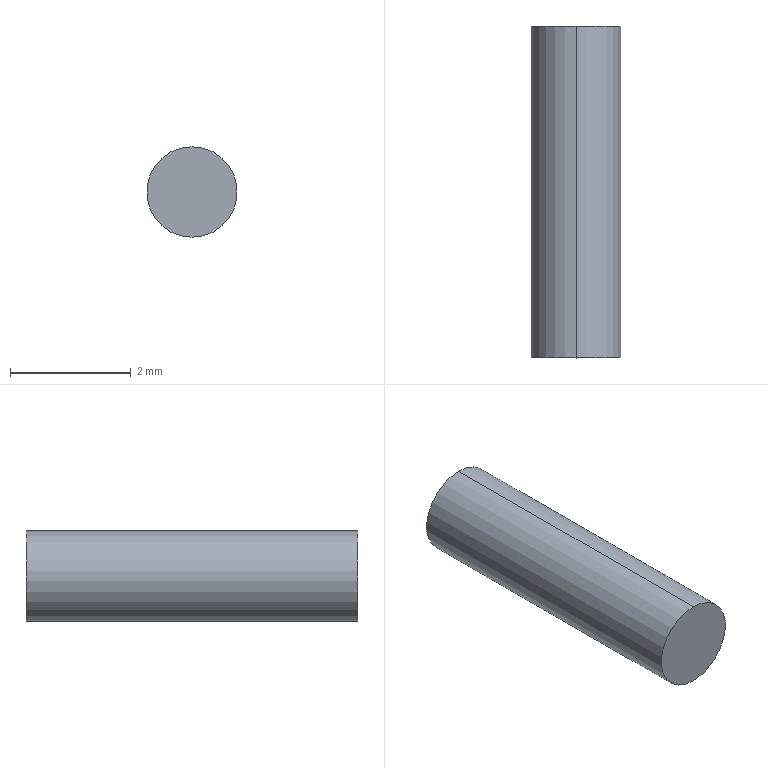Part | STEP file | part 11.stp.STEP-264.STEP | 1 solid | 4 faces | box 1.5 x 5.5 x 1.5 mm | volume 9.719 mm3 | cylinder 2 | plane 2 | commonest cylinder face diameters 1.5 x2
STEP:
#1=CARTESIAN_POINT('',(429.94,12.75,-0.75));
#2=VERTEX_POINT('',#1);
#3=CARTESIAN_POINT('',(429.94,12.75,0.75));
#4=VERTEX_POINT('',#3);
#5=CARTESIAN_POINT('',(429.94,12.75,0.));
#6=DIRECTION('',(0.,-1.,0.));
#7=DIRECTION('',(0.,0.,-1.));
#8=AXIS2_PLACEMENT_3D('',#5,#6,#7);
#9=CIRCLE('',#8,0.75);
#10=EDGE_CURVE('',#2,#4,#9,.T.);
#11=ORIENTED_EDGE('',*,*,#10,.T.);
#12=CARTESIAN_POINT('',(429.94,7.25,0.75));
#13=VERTEX_POINT('',#12);
#14=CARTESIAN_POINT('',(429.94,8.875,0.75));
#15=DIRECTION('',(0.,-1.,0.));
#16=VECTOR('',#15,1000.);
#17=LINE('',#14,#16);
#18=EDGE_CURVE('',#4,#13,#17,.T.);
#19=ORIENTED_EDGE('',*,*,#18,.T.);
#20=CARTESIAN_POINT('',(429.94,7.25,-0.75));
#21=VERTEX_POINT('',#20);
#22=CARTESIAN_POINT('',(429.94,7.25,0.));
#23=DIRECTION('',(0.,-1.,0.));
#24=DIRECTION('',(0.,0.,-1.));
#25=AXIS2_PLACEMENT_3D('',#22,#23,#24);
#26=CIRCLE('',#25,0.75);
#27=EDGE_CURVE('',#21,#13,#26,.T.);
#28=ORIENTED_EDGE('',*,*,#27,.F.);
#29=CARTESIAN_POINT('',(429.94,8.875,-0.75));
#30=DIRECTION('',(0.,-1.,0.));
#31=VECTOR('',#30,1000.);
#32=LINE('',#29,#31);
#33=EDGE_CURVE('',#2,#21,#32,.T.);
#34=ORIENTED_EDGE('',*,*,#33,.F.);
#35=EDGE_LOOP('',(#11,#19,#28,#34));
#36=FACE_OUTER_BOUND('',#35,.T.);
#37=CARTESIAN_POINT('',(429.94,8.875,0.));
#38=DIRECTION('',(0.,-1.,0.));
#39=DIRECTION('',(0.,0.,-1.));
#40=AXIS2_PLACEMENT_3D('',#37,#38,#39);
#41=CYLINDRICAL_SURFACE('',#40,0.75);
#42=ADVANCED_FACE('',(#36),#41,.T.);
#43=ORIENTED_EDGE('',*,*,#27,.T.);
#44=CARTESIAN_POINT('',(429.94,7.25,0.));
#45=DIRECTION('',(0.,-1.,0.));
#46=DIRECTION('',(0.,0.,-1.));
#47=AXIS2_PLACEMENT_3D('',#44,#45,#46);
#48=CIRCLE('',#47,0.75);
#49=EDGE_CURVE('',#13,#21,#48,.T.);
#50=ORIENTED_EDGE('',*,*,#49,.T.);
#51=EDGE_LOOP('',(#43,#50));
#52=FACE_OUTER_BOUND('',#51,.T.);
#53=CARTESIAN_POINT('',(429.94,7.25,0.));
#54=DIRECTION('',(0.,-1.,0.));
#55=DIRECTION('',(-1.,0.,0.));
#56=AXIS2_PLACEMENT_3D('',#53,#54,#55);
#57=PLANE('',#56);
#58=ADVANCED_FACE('',(#52),#57,.T.);
#59=ORIENTED_EDGE('',*,*,#18,.F.);
#60=CARTESIAN_POINT('',(429.94,12.75,0.));
#61=DIRECTION('',(0.,-1.,0.));
#62=DIRECTION('',(0.,0.,-1.));
#63=AXIS2_PLACEMENT_3D('',#60,#61,#62);
#64=CIRCLE('',#63,0.75);
#65=EDGE_CURVE('',#4,#2,#64,.T.);
#66=ORIENTED_EDGE('',*,*,#65,.T.);
#67=ORIENTED_EDGE('',*,*,#33,.T.);
#68=ORIENTED_EDGE('',*,*,#49,.F.);
#69=EDGE_LOOP('',(#59,#66,#67,#68));
#70=FACE_OUTER_BOUND('',#69,.T.);
#71=CARTESIAN_POINT('',(429.94,8.875,0.));
#72=DIRECTION('',(0.,-1.,0.));
#73=DIRECTION('',(0.,0.,-1.));
#74=AXIS2_PLACEMENT_3D('',#71,#72,#73);
#75=CYLINDRICAL_SURFACE('',#74,0.75);
#76=ADVANCED_FACE('',(#70),#75,.T.);
#77=ORIENTED_EDGE('',*,*,#10,.F.);
#78=ORIENTED_EDGE('',*,*,#65,.F.);
#79=EDGE_LOOP('',(#77,#78));
#80=FACE_OUTER_BOUND('',#79,.T.);
#81=CARTESIAN_POINT('',(430.69,12.75,0.));
#82=DIRECTION('',(0.,1.,0.));
#83=DIRECTION('',(0.,0.,-1.));
#84=AXIS2_PLACEMENT_3D('',#81,#82,#83);
#85=PLANE('',#84);
#86=ADVANCED_FACE('',(#80),#85,.T.);
#87=CLOSED_SHELL('',(#42,#58,#76,#86));
#88=MANIFOLD_SOLID_BREP('',#87);
#89=CARTESIAN_POINT('',(0.,0.,0.));
#90=DIRECTION('',(0.,0.,1.));
#91=DIRECTION('',(1.,0.,0.));
#92=AXIS2_PLACEMENT_3D('',#89,#90,#91);
#93=(LENGTH_UNIT()NAMED_UNIT(*)SI_UNIT(.MILLI.,.METRE.));
#94=UNCERTAINTY_MEASURE_WITH_UNIT(LENGTH_MEASURE(0.00001),#93,'','');
#95=(NAMED_UNIT(*)PLANE_ANGLE_UNIT()SI_UNIT($,.RADIAN.));
#96=(NAMED_UNIT(*)SI_UNIT($,.STERADIAN.)SOLID_ANGLE_UNIT());
#97=(GEOMETRIC_REPRESENTATION_CONTEXT(3)GLOBAL_UNCERTAINTY_ASSIGNED_CONTEXT((#94))GLOBAL_UNIT_ASSIGNED_CONTEXT((#93,#95,#96))REPRESENTATION_CONTEXT('',''));
#98=ADVANCED_BREP_SHAPE_REPRESENTATION('',(#88,#92),#97);